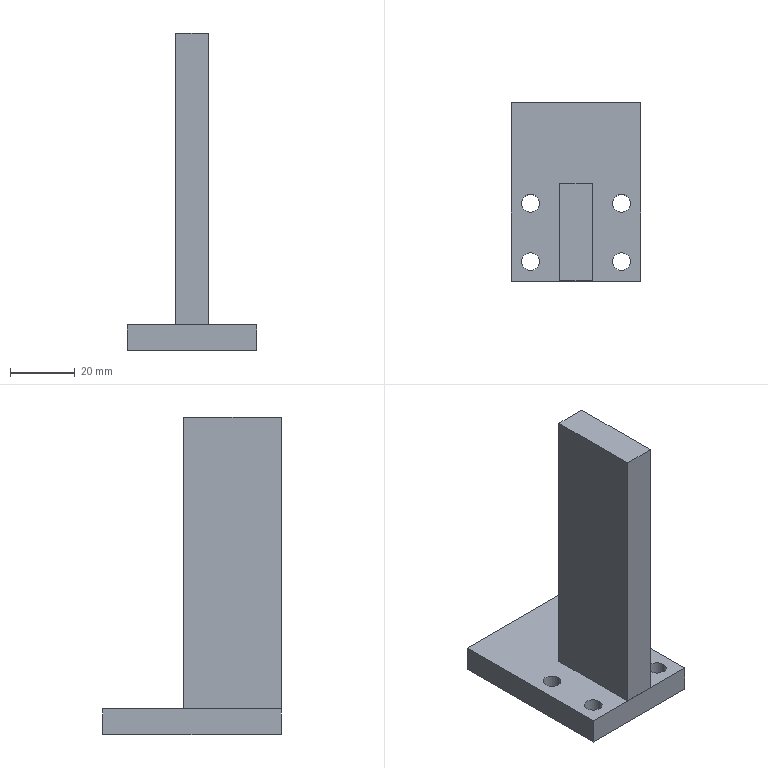Part | STEP file | X77-04020 | 2 solids | 20 faces | box 40 x 55 x 98 mm | volume 43840 mm3 | plane 12 | cylinder 8 | commonest cylinder face diameters 5.5 x8
STEP:
#1=CARTESIAN_POINT('',(338.059,99.5,0.));
#2=VERTEX_POINT('',#1);
#3=CARTESIAN_POINT('',(338.059,129.5,0.));
#4=VERTEX_POINT('',#3);
#5=CARTESIAN_POINT('',(338.059,99.5,0.));
#6=DIRECTION('',(0.,1.,0.));
#7=VECTOR('',#6,1000.);
#8=LINE('',#5,#7);
#9=EDGE_CURVE('',#2,#4,#8,.T.);
#10=ORIENTED_EDGE('',*,*,#9,.T.);
#11=CARTESIAN_POINT('',(338.059,129.5,90.));
#12=VERTEX_POINT('',#11);
#13=CARTESIAN_POINT('',(338.059,129.5,90.));
#14=DIRECTION('',(0.,0.,-1.));
#15=VECTOR('',#14,1000.);
#16=LINE('',#13,#15);
#17=EDGE_CURVE('',#12,#4,#16,.T.);
#18=ORIENTED_EDGE('',*,*,#17,.F.);
#19=CARTESIAN_POINT('',(338.059,99.5,90.));
#20=VERTEX_POINT('',#19);
#21=CARTESIAN_POINT('',(338.059,99.5,90.));
#22=DIRECTION('',(0.,1.,0.));
#23=VECTOR('',#22,1000.);
#24=LINE('',#21,#23);
#25=EDGE_CURVE('',#20,#12,#24,.T.);
#26=ORIENTED_EDGE('',*,*,#25,.F.);
#27=CARTESIAN_POINT('',(338.059,99.5,90.));
#28=DIRECTION('',(0.,0.,-1.));
#29=VECTOR('',#28,1000.);
#30=LINE('',#27,#29);
#31=EDGE_CURVE('',#20,#2,#30,.T.);
#32=ORIENTED_EDGE('',*,*,#31,.T.);
#33=EDGE_LOOP('',(#10,#18,#26,#32));
#34=FACE_OUTER_BOUND('',#33,.T.);
#35=CARTESIAN_POINT('',(338.059,99.5,90.));
#36=DIRECTION('',(-1.,0.,0.));
#37=DIRECTION('',(0.,0.,1.));
#38=AXIS2_PLACEMENT_3D('',#35,#36,#37);
#39=PLANE('',#38);
#40=ADVANCED_FACE('',(#34),#39,.F.);
#41=CARTESIAN_POINT('',(328.059,129.5,0.));
#42=VERTEX_POINT('',#41);
#43=CARTESIAN_POINT('',(328.059,129.5,0.));
#44=DIRECTION('',(-1.,0.,0.));
#45=VECTOR('',#44,1000.);
#46=LINE('',#43,#45);
#47=EDGE_CURVE('',#4,#42,#46,.T.);
#48=ORIENTED_EDGE('',*,*,#47,.T.);
#49=CARTESIAN_POINT('',(328.059,129.5,90.));
#50=VERTEX_POINT('',#49);
#51=CARTESIAN_POINT('',(328.059,129.5,90.));
#52=DIRECTION('',(0.,0.,-1.));
#53=VECTOR('',#52,1000.);
#54=LINE('',#51,#53);
#55=EDGE_CURVE('',#50,#42,#54,.T.);
#56=ORIENTED_EDGE('',*,*,#55,.F.);
#57=CARTESIAN_POINT('',(328.059,129.5,90.));
#58=DIRECTION('',(-1.,0.,0.));
#59=VECTOR('',#58,1000.);
#60=LINE('',#57,#59);
#61=EDGE_CURVE('',#12,#50,#60,.T.);
#62=ORIENTED_EDGE('',*,*,#61,.F.);
#63=ORIENTED_EDGE('',*,*,#17,.T.);
#64=EDGE_LOOP('',(#48,#56,#62,#63));
#65=FACE_OUTER_BOUND('',#64,.T.);
#66=CARTESIAN_POINT('',(328.059,129.5,90.));
#67=DIRECTION('',(0.,-1.,0.));
#68=DIRECTION('',(0.,0.,-1.));
#69=AXIS2_PLACEMENT_3D('',#66,#67,#68);
#70=PLANE('',#69);
#71=ADVANCED_FACE('',(#65),#70,.F.);
#72=CARTESIAN_POINT('',(328.059,99.5,0.));
#73=VERTEX_POINT('',#72);
#74=CARTESIAN_POINT('',(328.059,99.5,0.));
#75=DIRECTION('',(0.,-1.,0.));
#76=VECTOR('',#75,1000.);
#77=LINE('',#74,#76);
#78=EDGE_CURVE('',#42,#73,#77,.T.);
#79=ORIENTED_EDGE('',*,*,#78,.T.);
#80=CARTESIAN_POINT('',(328.059,99.5,90.));
#81=VERTEX_POINT('',#80);
#82=CARTESIAN_POINT('',(328.059,99.5,90.));
#83=DIRECTION('',(0.,0.,-1.));
#84=VECTOR('',#83,1000.);
#85=LINE('',#82,#84);
#86=EDGE_CURVE('',#81,#73,#85,.T.);
#87=ORIENTED_EDGE('',*,*,#86,.F.);
#88=CARTESIAN_POINT('',(328.059,99.5,90.));
#89=DIRECTION('',(0.,-1.,0.));
#90=VECTOR('',#89,1000.);
#91=LINE('',#88,#90);
#92=EDGE_CURVE('',#50,#81,#91,.T.);
#93=ORIENTED_EDGE('',*,*,#92,.F.);
#94=ORIENTED_EDGE('',*,*,#55,.T.);
#95=EDGE_LOOP('',(#79,#87,#93,#94));
#96=FACE_OUTER_BOUND('',#95,.T.);
#97=CARTESIAN_POINT('',(328.059,99.5,90.));
#98=DIRECTION('',(1.,0.,0.));
#99=DIRECTION('',(0.,0.,-1.));
#100=AXIS2_PLACEMENT_3D('',#97,#98,#99);
#101=PLANE('',#100);
#102=ADVANCED_FACE('',(#96),#101,.F.);
#103=CARTESIAN_POINT('',(328.059,99.5,0.));
#104=DIRECTION('',(1.,0.,0.));
#105=VECTOR('',#104,1000.);
#106=LINE('',#103,#105);
#107=EDGE_CURVE('',#73,#2,#106,.T.);
#108=ORIENTED_EDGE('',*,*,#107,.T.);
#109=ORIENTED_EDGE('',*,*,#31,.F.);
#110=CARTESIAN_POINT('',(328.059,99.5,90.));
#111=DIRECTION('',(1.,0.,0.));
#112=VECTOR('',#111,1000.);
#113=LINE('',#110,#112);
#114=EDGE_CURVE('',#81,#20,#113,.T.);
#115=ORIENTED_EDGE('',*,*,#114,.F.);
#116=ORIENTED_EDGE('',*,*,#86,.T.);
#117=EDGE_LOOP('',(#108,#109,#115,#116));
#118=FACE_OUTER_BOUND('',#117,.T.);
#119=CARTESIAN_POINT('',(328.059,99.5,90.));
#120=DIRECTION('',(0.,1.,0.));
#121=DIRECTION('',(0.,0.,1.));
#122=AXIS2_PLACEMENT_3D('',#119,#120,#121);
#123=PLANE('',#122);
#124=ADVANCED_FACE('',(#118),#123,.F.);
#125=ORIENTED_EDGE('',*,*,#25,.T.);
#126=ORIENTED_EDGE('',*,*,#61,.T.);
#127=ORIENTED_EDGE('',*,*,#92,.T.);
#128=ORIENTED_EDGE('',*,*,#114,.T.);
#129=EDGE_LOOP('',(#125,#126,#127,#128));
#130=FACE_OUTER_BOUND('',#129,.T.);
#131=CARTESIAN_POINT('',(338.059,129.5,90.));
#132=DIRECTION('',(0.,0.,-1.));
#133=DIRECTION('',(-1.,0.,0.));
#134=AXIS2_PLACEMENT_3D('',#131,#132,#133);
#135=PLANE('',#134);
#136=ADVANCED_FACE('',(#130),#135,.F.);
#137=ORIENTED_EDGE('',*,*,#9,.F.);
#138=ORIENTED_EDGE('',*,*,#107,.F.);
#139=ORIENTED_EDGE('',*,*,#78,.F.);
#140=ORIENTED_EDGE('',*,*,#47,.F.);
#141=EDGE_LOOP('',(#137,#138,#139,#140));
#142=FACE_OUTER_BOUND('',#141,.T.);
#143=CARTESIAN_POINT('',(338.059,129.5,0.));
#144=DIRECTION('',(0.,0.,-1.));
#145=DIRECTION('',(-1.,0.,0.));
#146=AXIS2_PLACEMENT_3D('',#143,#144,#145);
#147=PLANE('',#146);
#148=ADVANCED_FACE('',(#142),#147,.T.);
#149=CLOSED_SHELL('',(#40,#71,#102,#124,#136,#148));
#150=MANIFOLD_SOLID_BREP('',#149);
#151=CARTESIAN_POINT('',(316.309,123.5,-8.));
#152=VERTEX_POINT('',#151);
#153=CARTESIAN_POINT('',(321.809,123.5,-8.));
#154=VERTEX_POINT('',#153);
#155=CARTESIAN_POINT('',(319.059,123.5,-8.));
#156=DIRECTION('',(0.,0.,1.));
#157=DIRECTION('',(1.,0.,0.));
#158=AXIS2_PLACEMENT_3D('',#155,#156,#157);
#159=CIRCLE('',#158,2.75);
#160=EDGE_CURVE('',#152,#154,#159,.T.);
#161=ORIENTED_EDGE('',*,*,#160,.F.);
#162=CARTESIAN_POINT('',(316.309,123.5,0.));
#163=VERTEX_POINT('',#162);
#164=CARTESIAN_POINT('',(316.309,123.5,0.));
#165=DIRECTION('',(0.,0.,1.));
#166=VECTOR('',#165,1000.);
#167=LINE('',#164,#166);
#168=EDGE_CURVE('',#152,#163,#167,.T.);
#169=ORIENTED_EDGE('',*,*,#168,.T.);
#170=CARTESIAN_POINT('',(321.809,123.5,0.));
#171=VERTEX_POINT('',#170);
#172=CARTESIAN_POINT('',(319.059,123.5,0.));
#173=DIRECTION('',(0.,0.,1.));
#174=DIRECTION('',(1.,0.,0.));
#175=AXIS2_PLACEMENT_3D('',#172,#173,#174);
#176=CIRCLE('',#175,2.75);
#177=EDGE_CURVE('',#163,#171,#176,.T.);
#178=ORIENTED_EDGE('',*,*,#177,.T.);
#179=CARTESIAN_POINT('',(321.809,123.5,0.));
#180=DIRECTION('',(0.,0.,1.));
#181=VECTOR('',#180,1000.);
#182=LINE('',#179,#181);
#183=EDGE_CURVE('',#154,#171,#182,.T.);
#184=ORIENTED_EDGE('',*,*,#183,.F.);
#185=EDGE_LOOP('',(#161,#169,#178,#184));
#186=FACE_OUTER_BOUND('',#185,.T.);
#187=CARTESIAN_POINT('',(319.059,123.5,0.));
#188=DIRECTION('',(0.,0.,1.));
#189=DIRECTION('',(1.,0.,0.));
#190=AXIS2_PLACEMENT_3D('',#187,#188,#189);
#191=CYLINDRICAL_SURFACE('',#190,2.75);
#192=ADVANCED_FACE('',(#186),#191,.F.);
#193=CARTESIAN_POINT('',(344.309,123.5,-8.));
#194=VERTEX_POINT('',#193);
#195=CARTESIAN_POINT('',(349.809,123.5,-8.));
#196=VERTEX_POINT('',#195);
#197=CARTESIAN_POINT('',(347.059,123.5,-8.));
#198=DIRECTION('',(0.,0.,1.));
#199=DIRECTION('',(1.,0.,0.));
#200=AXIS2_PLACEMENT_3D('',#197,#198,#199);
#201=CIRCLE('',#200,2.75);
#202=EDGE_CURVE('',#194,#196,#201,.T.);
#203=ORIENTED_EDGE('',*,*,#202,.F.);
#204=CARTESIAN_POINT('',(344.309,123.5,0.));
#205=VERTEX_POINT('',#204);
#206=CARTESIAN_POINT('',(344.309,123.5,0.));
#207=DIRECTION('',(0.,0.,1.));
#208=VECTOR('',#207,1000.);
#209=LINE('',#206,#208);
#210=EDGE_CURVE('',#194,#205,#209,.T.);
#211=ORIENTED_EDGE('',*,*,#210,.T.);
#212=CARTESIAN_POINT('',(349.809,123.5,0.));
#213=VERTEX_POINT('',#212);
#214=CARTESIAN_POINT('',(347.059,123.5,0.));
#215=DIRECTION('',(0.,0.,1.));
#216=DIRECTION('',(1.,0.,0.));
#217=AXIS2_PLACEMENT_3D('',#214,#215,#216);
#218=CIRCLE('',#217,2.75);
#219=EDGE_CURVE('',#205,#213,#218,.T.);
#220=ORIENTED_EDGE('',*,*,#219,.T.);
#221=CARTESIAN_POINT('',(349.809,123.5,0.));
#222=DIRECTION('',(0.,0.,1.));
#223=VECTOR('',#222,1000.);
#224=LINE('',#221,#223);
#225=EDGE_CURVE('',#196,#213,#224,.T.);
#226=ORIENTED_EDGE('',*,*,#225,.F.);
#227=EDGE_LOOP('',(#203,#211,#220,#226));
#228=FACE_OUTER_BOUND('',#227,.T.);
#229=CARTESIAN_POINT('',(347.059,123.5,0.));
#230=DIRECTION('',(0.,0.,1.));
#231=DIRECTION('',(1.,0.,0.));
#232=AXIS2_PLACEMENT_3D('',#229,#230,#231);
#233=CYLINDRICAL_SURFACE('',#232,2.75);
#234=ADVANCED_FACE('',(#228),#233,.F.);
#235=CARTESIAN_POINT('',(316.309,105.5,-8.));
#236=VERTEX_POINT('',#235);
#237=CARTESIAN_POINT('',(321.809,105.5,-8.));
#238=VERTEX_POINT('',#237);
#239=CARTESIAN_POINT('',(319.059,105.5,-8.));
#240=DIRECTION('',(0.,0.,1.));
#241=DIRECTION('',(1.,0.,0.));
#242=AXIS2_PLACEMENT_3D('',#239,#240,#241);
#243=CIRCLE('',#242,2.75);
#244=EDGE_CURVE('',#236,#238,#243,.T.);
#245=ORIENTED_EDGE('',*,*,#244,.F.);
#246=CARTESIAN_POINT('',(316.309,105.5,0.));
#247=VERTEX_POINT('',#246);
#248=CARTESIAN_POINT('',(316.309,105.5,0.));
#249=DIRECTION('',(0.,0.,1.));
#250=VECTOR('',#249,1000.);
#251=LINE('',#248,#250);
#252=EDGE_CURVE('',#236,#247,#251,.T.);
#253=ORIENTED_EDGE('',*,*,#252,.T.);
#254=CARTESIAN_POINT('',(321.809,105.5,0.));
#255=VERTEX_POINT('',#254);
#256=CARTESIAN_POINT('',(319.059,105.5,0.));
#257=DIRECTION('',(0.,0.,1.));
#258=DIRECTION('',(1.,0.,0.));
#259=AXIS2_PLACEMENT_3D('',#256,#257,#258);
#260=CIRCLE('',#259,2.75);
#261=EDGE_CURVE('',#247,#255,#260,.T.);
#262=ORIENTED_EDGE('',*,*,#261,.T.);
#263=CARTESIAN_POINT('',(321.809,105.5,0.));
#264=DIRECTION('',(0.,0.,1.));
#265=VECTOR('',#264,1000.);
#266=LINE('',#263,#265);
#267=EDGE_CURVE('',#238,#255,#266,.T.);
#268=ORIENTED_EDGE('',*,*,#267,.F.);
#269=EDGE_LOOP('',(#245,#253,#262,#268));
#270=FACE_OUTER_BOUND('',#269,.T.);
#271=CARTESIAN_POINT('',(319.059,105.5,0.));
#272=DIRECTION('',(0.,0.,1.));
#273=DIRECTION('',(1.,0.,0.));
#274=AXIS2_PLACEMENT_3D('',#271,#272,#273);
#275=CYLINDRICAL_SURFACE('',#274,2.75);
#276=ADVANCED_FACE('',(#270),#275,.F.);
#277=CARTESIAN_POINT('',(344.309,105.5,-8.));
#278=VERTEX_POINT('',#277);
#279=CARTESIAN_POINT('',(349.809,105.5,-8.));
#280=VERTEX_POINT('',#279);
#281=CARTESIAN_POINT('',(347.059,105.5,-8.));
#282=DIRECTION('',(0.,0.,1.));
#283=DIRECTION('',(1.,0.,0.));
#284=AXIS2_PLACEMENT_3D('',#281,#282,#283);
#285=CIRCLE('',#284,2.75);
#286=EDGE_CURVE('',#278,#280,#285,.T.);
#287=ORIENTED_EDGE('',*,*,#286,.F.);
#288=CARTESIAN_POINT('',(344.309,105.5,0.));
#289=VERTEX_POINT('',#288);
#290=CARTESIAN_POINT('',(344.309,105.5,0.));
#291=DIRECTION('',(0.,0.,1.));
#292=VECTOR('',#291,1000.);
#293=LINE('',#290,#292);
#294=EDGE_CURVE('',#278,#289,#293,.T.);
#295=ORIENTED_EDGE('',*,*,#294,.T.);
#296=CARTESIAN_POINT('',(349.809,105.5,0.));
#297=VERTEX_POINT('',#296);
#298=CARTESIAN_POINT('',(347.059,105.5,0.));
#299=DIRECTION('',(0.,0.,1.));
#300=DIRECTION('',(1.,0.,0.));
#301=AXIS2_PLACEMENT_3D('',#298,#299,#300);
#302=CIRCLE('',#301,2.75);
#303=EDGE_CURVE('',#289,#297,#302,.T.);
#304=ORIENTED_EDGE('',*,*,#303,.T.);
#305=CARTESIAN_POINT('',(349.809,105.5,0.));
#306=DIRECTION('',(0.,0.,1.));
#307=VECTOR('',#306,1000.);
#308=LINE('',#305,#307);
#309=EDGE_CURVE('',#280,#297,#308,.T.);
#310=ORIENTED_EDGE('',*,*,#309,.F.);
#311=EDGE_LOOP('',(#287,#295,#304,#310));
#312=FACE_OUTER_BOUND('',#311,.T.);
#313=CARTESIAN_POINT('',(347.059,105.5,0.));
#314=DIRECTION('',(0.,0.,1.));
#315=DIRECTION('',(1.,0.,0.));
#316=AXIS2_PLACEMENT_3D('',#313,#314,#315);
#317=CYLINDRICAL_SURFACE('',#316,2.75);
#318=ADVANCED_FACE('',(#312),#317,.F.);
#319=CARTESIAN_POINT('',(313.059,99.5,0.));
#320=VERTEX_POINT('',#319);
#321=CARTESIAN_POINT('',(313.059,154.5,0.));
#322=VERTEX_POINT('',#321);
#323=CARTESIAN_POINT('',(313.059,99.5,0.));
#324=DIRECTION('',(0.,1.,0.));
#325=VECTOR('',#324,1000.);
#326=LINE('',#323,#325);
#327=EDGE_CURVE('',#320,#322,#326,.T.);
#328=ORIENTED_EDGE('',*,*,#327,.T.);
#329=CARTESIAN_POINT('',(313.059,154.5,-8.));
#330=VERTEX_POINT('',#329);
#331=CARTESIAN_POINT('',(313.059,154.5,0.));
#332=DIRECTION('',(0.,0.,1.));
#333=VECTOR('',#332,1000.);
#334=LINE('',#331,#333);
#335=EDGE_CURVE('',#330,#322,#334,.T.);
#336=ORIENTED_EDGE('',*,*,#335,.F.);
#337=CARTESIAN_POINT('',(313.059,99.5,-8.));
#338=VERTEX_POINT('',#337);
#339=CARTESIAN_POINT('',(313.059,99.5,-8.));
#340=DIRECTION('',(0.,1.,0.));
#341=VECTOR('',#340,1000.);
#342=LINE('',#339,#341);
#343=EDGE_CURVE('',#338,#330,#342,.T.);
#344=ORIENTED_EDGE('',*,*,#343,.F.);
#345=CARTESIAN_POINT('',(313.059,99.5,-8.));
#346=DIRECTION('',(0.,0.,1.));
#347=VECTOR('',#346,1000.);
#348=LINE('',#345,#347);
#349=EDGE_CURVE('',#338,#320,#348,.T.);
#350=ORIENTED_EDGE('',*,*,#349,.T.);
#351=EDGE_LOOP('',(#328,#336,#344,#350));
#352=FACE_OUTER_BOUND('',#351,.T.);
#353=CARTESIAN_POINT('',(313.059,99.5,-8.));
#354=DIRECTION('',(1.,0.,0.));
#355=DIRECTION('',(0.,0.,-1.));
#356=AXIS2_PLACEMENT_3D('',#353,#354,#355);
#357=PLANE('',#356);
#358=ADVANCED_FACE('',(#352),#357,.F.);
#359=CARTESIAN_POINT('',(353.059,154.5,0.));
#360=VERTEX_POINT('',#359);
#361=CARTESIAN_POINT('',(353.059,99.5,0.));
#362=VERTEX_POINT('',#361);
#363=CARTESIAN_POINT('',(353.059,99.5,0.));
#364=DIRECTION('',(0.,-1.,0.));
#365=VECTOR('',#364,1000.);
#366=LINE('',#363,#365);
#367=EDGE_CURVE('',#360,#362,#366,.T.);
#368=ORIENTED_EDGE('',*,*,#367,.T.);
#369=CARTESIAN_POINT('',(353.059,99.5,-8.));
#370=VERTEX_POINT('',#369);
#371=CARTESIAN_POINT('',(353.059,99.5,-8.));
#372=DIRECTION('',(0.,0.,1.));
#373=VECTOR('',#372,1000.);
#374=LINE('',#371,#373);
#375=EDGE_CURVE('',#370,#362,#374,.T.);
#376=ORIENTED_EDGE('',*,*,#375,.F.);
#377=CARTESIAN_POINT('',(353.059,154.5,-8.));
#378=VERTEX_POINT('',#377);
#379=CARTESIAN_POINT('',(353.059,99.5,-8.));
#380=DIRECTION('',(0.,-1.,0.));
#381=VECTOR('',#380,1000.);
#382=LINE('',#379,#381);
#383=EDGE_CURVE('',#378,#370,#382,.T.);
#384=ORIENTED_EDGE('',*,*,#383,.F.);
#385=CARTESIAN_POINT('',(353.059,154.5,0.));
#386=DIRECTION('',(0.,0.,-1.));
#387=VECTOR('',#386,1000.);
#388=LINE('',#385,#387);
#389=EDGE_CURVE('',#360,#378,#388,.T.);
#390=ORIENTED_EDGE('',*,*,#389,.F.);
#391=EDGE_LOOP('',(#368,#376,#384,#390));
#392=FACE_OUTER_BOUND('',#391,.T.);
#393=CARTESIAN_POINT('',(353.059,99.5,-8.));
#394=DIRECTION('',(-1.,0.,0.));
#395=DIRECTION('',(0.,0.,1.));
#396=AXIS2_PLACEMENT_3D('',#393,#394,#395);
#397=PLANE('',#396);
#398=ADVANCED_FACE('',(#392),#397,.F.);
#399=CARTESIAN_POINT('',(353.059,99.5,0.));
#400=DIRECTION('',(-1.,0.,0.));
#401=VECTOR('',#400,1000.);
#402=LINE('',#399,#401);
#403=EDGE_CURVE('',#362,#320,#402,.T.);
#404=ORIENTED_EDGE('',*,*,#403,.T.);
#405=ORIENTED_EDGE('',*,*,#349,.F.);
#406=CARTESIAN_POINT('',(353.059,99.5,-8.));
#407=DIRECTION('',(-1.,0.,0.));
#408=VECTOR('',#407,1000.);
#409=LINE('',#406,#408);
#410=EDGE_CURVE('',#370,#338,#409,.T.);
#411=ORIENTED_EDGE('',*,*,#410,.F.);
#412=ORIENTED_EDGE('',*,*,#375,.T.);
#413=EDGE_LOOP('',(#404,#405,#411,#412));
#414=FACE_OUTER_BOUND('',#413,.T.);
#415=CARTESIAN_POINT('',(353.059,99.5,-8.));
#416=DIRECTION('',(0.,1.,0.));
#417=DIRECTION('',(0.,0.,1.));
#418=AXIS2_PLACEMENT_3D('',#415,#416,#417);
#419=PLANE('',#418);
#420=ADVANCED_FACE('',(#414),#419,.F.);
#421=CARTESIAN_POINT('',(319.059,123.5,-8.));
#422=DIRECTION('',(0.,0.,1.));
#423=DIRECTION('',(1.,0.,0.));
#424=AXIS2_PLACEMENT_3D('',#421,#422,#423);
#425=CIRCLE('',#424,2.75);
#426=EDGE_CURVE('',#154,#152,#425,.T.);
#427=ORIENTED_EDGE('',*,*,#426,.T.);
#428=ORIENTED_EDGE('',*,*,#160,.T.);
#429=EDGE_LOOP('',(#427,#428));
#430=FACE_BOUND('',#429,.T.);
#431=CARTESIAN_POINT('',(347.059,123.5,-8.));
#432=DIRECTION('',(0.,0.,1.));
#433=DIRECTION('',(1.,0.,0.));
#434=AXIS2_PLACEMENT_3D('',#431,#432,#433);
#435=CIRCLE('',#434,2.75);
#436=EDGE_CURVE('',#196,#194,#435,.T.);
#437=ORIENTED_EDGE('',*,*,#436,.T.);
#438=ORIENTED_EDGE('',*,*,#202,.T.);
#439=EDGE_LOOP('',(#437,#438));
#440=FACE_BOUND('',#439,.T.);
#441=CARTESIAN_POINT('',(319.059,105.5,-8.));
#442=DIRECTION('',(0.,0.,1.));
#443=DIRECTION('',(1.,0.,0.));
#444=AXIS2_PLACEMENT_3D('',#441,#442,#443);
#445=CIRCLE('',#444,2.75);
#446=EDGE_CURVE('',#238,#236,#445,.T.);
#447=ORIENTED_EDGE('',*,*,#446,.T.);
#448=ORIENTED_EDGE('',*,*,#244,.T.);
#449=EDGE_LOOP('',(#447,#448));
#450=FACE_BOUND('',#449,.T.);
#451=CARTESIAN_POINT('',(347.059,105.5,-8.));
#452=DIRECTION('',(0.,0.,1.));
#453=DIRECTION('',(1.,0.,0.));
#454=AXIS2_PLACEMENT_3D('',#451,#452,#453);
#455=CIRCLE('',#454,2.75);
#456=EDGE_CURVE('',#280,#278,#455,.T.);
#457=ORIENTED_EDGE('',*,*,#456,.T.);
#458=ORIENTED_EDGE('',*,*,#286,.T.);
#459=EDGE_LOOP('',(#457,#458));
#460=FACE_BOUND('',#459,.T.);
#461=ORIENTED_EDGE('',*,*,#343,.T.);
#462=CARTESIAN_POINT('',(313.059,154.5,-8.));
#463=DIRECTION('',(-1.,0.,0.));
#464=VECTOR('',#463,1000.);
#465=LINE('',#462,#464);
#466=EDGE_CURVE('',#378,#330,#465,.T.);
#467=ORIENTED_EDGE('',*,*,#466,.F.);
#468=ORIENTED_EDGE('',*,*,#383,.T.);
#469=ORIENTED_EDGE('',*,*,#410,.T.);
#470=EDGE_LOOP('',(#461,#467,#468,#469));
#471=FACE_OUTER_BOUND('',#470,.T.);
#472=CARTESIAN_POINT('',(313.059,129.5,-8.));
#473=DIRECTION('',(0.,0.,1.));
#474=DIRECTION('',(1.,0.,0.));
#475=AXIS2_PLACEMENT_3D('',#472,#473,#474);
#476=PLANE('',#475);
#477=ADVANCED_FACE('',(#430,#440,#450,#460,#471),#476,.F.);
#478=CARTESIAN_POINT('',(319.059,123.5,0.));
#479=DIRECTION('',(0.,0.,1.));
#480=DIRECTION('',(1.,0.,0.));
#481=AXIS2_PLACEMENT_3D('',#478,#479,#480);
#482=CIRCLE('',#481,2.75);
#483=EDGE_CURVE('',#171,#163,#482,.T.);
#484=ORIENTED_EDGE('',*,*,#483,.F.);
#485=ORIENTED_EDGE('',*,*,#177,.F.);
#486=EDGE_LOOP('',(#484,#485));
#487=FACE_BOUND('',#486,.T.);
#488=CARTESIAN_POINT('',(347.059,123.5,0.));
#489=DIRECTION('',(0.,0.,1.));
#490=DIRECTION('',(1.,0.,0.));
#491=AXIS2_PLACEMENT_3D('',#488,#489,#490);
#492=CIRCLE('',#491,2.75);
#493=EDGE_CURVE('',#213,#205,#492,.T.);
#494=ORIENTED_EDGE('',*,*,#493,.F.);
#495=ORIENTED_EDGE('',*,*,#219,.F.);
#496=EDGE_LOOP('',(#494,#495));
#497=FACE_BOUND('',#496,.T.);
#498=CARTESIAN_POINT('',(319.059,105.5,0.));
#499=DIRECTION('',(0.,0.,1.));
#500=DIRECTION('',(1.,0.,0.));
#501=AXIS2_PLACEMENT_3D('',#498,#499,#500);
#502=CIRCLE('',#501,2.75);
#503=EDGE_CURVE('',#255,#247,#502,.T.);
#504=ORIENTED_EDGE('',*,*,#503,.F.);
#505=ORIENTED_EDGE('',*,*,#261,.F.);
#506=EDGE_LOOP('',(#504,#505));
#507=FACE_BOUND('',#506,.T.);
#508=CARTESIAN_POINT('',(347.059,105.5,0.));
#509=DIRECTION('',(0.,0.,1.));
#510=DIRECTION('',(1.,0.,0.));
#511=AXIS2_PLACEMENT_3D('',#508,#509,#510);
#512=CIRCLE('',#511,2.75);
#513=EDGE_CURVE('',#297,#289,#512,.T.);
#514=ORIENTED_EDGE('',*,*,#513,.F.);
#515=ORIENTED_EDGE('',*,*,#303,.F.);
#516=EDGE_LOOP('',(#514,#515));
#517=FACE_BOUND('',#516,.T.);
#518=ORIENTED_EDGE('',*,*,#327,.F.);
#519=ORIENTED_EDGE('',*,*,#403,.F.);
#520=ORIENTED_EDGE('',*,*,#367,.F.);
#521=CARTESIAN_POINT('',(313.059,154.5,0.));
#522=DIRECTION('',(1.,0.,0.));
#523=VECTOR('',#522,1000.);
#524=LINE('',#521,#523);
#525=EDGE_CURVE('',#322,#360,#524,.T.);
#526=ORIENTED_EDGE('',*,*,#525,.F.);
#527=EDGE_LOOP('',(#518,#519,#520,#526));
#528=FACE_OUTER_BOUND('',#527,.T.);
#529=CARTESIAN_POINT('',(313.059,129.5,0.));
#530=DIRECTION('',(0.,0.,1.));
#531=DIRECTION('',(1.,0.,0.));
#532=AXIS2_PLACEMENT_3D('',#529,#530,#531);
#533=PLANE('',#532);
#534=ADVANCED_FACE('',(#487,#497,#507,#517,#528),#533,.T.);
#535=ORIENTED_EDGE('',*,*,#294,.F.);
#536=ORIENTED_EDGE('',*,*,#456,.F.);
#537=ORIENTED_EDGE('',*,*,#309,.T.);
#538=ORIENTED_EDGE('',*,*,#513,.T.);
#539=EDGE_LOOP('',(#535,#536,#537,#538));
#540=FACE_OUTER_BOUND('',#539,.T.);
#541=CARTESIAN_POINT('',(347.059,105.5,0.));
#542=DIRECTION('',(0.,0.,1.));
#543=DIRECTION('',(1.,0.,0.));
#544=AXIS2_PLACEMENT_3D('',#541,#542,#543);
#545=CYLINDRICAL_SURFACE('',#544,2.75);
#546=ADVANCED_FACE('',(#540),#545,.F.);
#547=ORIENTED_EDGE('',*,*,#252,.F.);
#548=ORIENTED_EDGE('',*,*,#446,.F.);
#549=ORIENTED_EDGE('',*,*,#267,.T.);
#550=ORIENTED_EDGE('',*,*,#503,.T.);
#551=EDGE_LOOP('',(#547,#548,#549,#550));
#552=FACE_OUTER_BOUND('',#551,.T.);
#553=CARTESIAN_POINT('',(319.059,105.5,0.));
#554=DIRECTION('',(0.,0.,1.));
#555=DIRECTION('',(1.,0.,0.));
#556=AXIS2_PLACEMENT_3D('',#553,#554,#555);
#557=CYLINDRICAL_SURFACE('',#556,2.75);
#558=ADVANCED_FACE('',(#552),#557,.F.);
#559=ORIENTED_EDGE('',*,*,#210,.F.);
#560=ORIENTED_EDGE('',*,*,#436,.F.);
#561=ORIENTED_EDGE('',*,*,#225,.T.);
#562=ORIENTED_EDGE('',*,*,#493,.T.);
#563=EDGE_LOOP('',(#559,#560,#561,#562));
#564=FACE_OUTER_BOUND('',#563,.T.);
#565=CARTESIAN_POINT('',(347.059,123.5,0.));
#566=DIRECTION('',(0.,0.,1.));
#567=DIRECTION('',(1.,0.,0.));
#568=AXIS2_PLACEMENT_3D('',#565,#566,#567);
#569=CYLINDRICAL_SURFACE('',#568,2.75);
#570=ADVANCED_FACE('',(#564),#569,.F.);
#571=ORIENTED_EDGE('',*,*,#168,.F.);
#572=ORIENTED_EDGE('',*,*,#426,.F.);
#573=ORIENTED_EDGE('',*,*,#183,.T.);
#574=ORIENTED_EDGE('',*,*,#483,.T.);
#575=EDGE_LOOP('',(#571,#572,#573,#574));
#576=FACE_OUTER_BOUND('',#575,.T.);
#577=CARTESIAN_POINT('',(319.059,123.5,0.));
#578=DIRECTION('',(0.,0.,1.));
#579=DIRECTION('',(1.,0.,0.));
#580=AXIS2_PLACEMENT_3D('',#577,#578,#579);
#581=CYLINDRICAL_SURFACE('',#580,2.75);
#582=ADVANCED_FACE('',(#576),#581,.F.);
#583=ORIENTED_EDGE('',*,*,#335,.T.);
#584=ORIENTED_EDGE('',*,*,#525,.T.);
#585=ORIENTED_EDGE('',*,*,#389,.T.);
#586=ORIENTED_EDGE('',*,*,#466,.T.);
#587=EDGE_LOOP('',(#583,#584,#585,#586));
#588=FACE_OUTER_BOUND('',#587,.T.);
#589=CARTESIAN_POINT('',(313.059,154.5,-8.));
#590=DIRECTION('',(0.,-1.,0.));
#591=DIRECTION('',(0.,0.,-1.));
#592=AXIS2_PLACEMENT_3D('',#589,#590,#591);
#593=PLANE('',#592);
#594=ADVANCED_FACE('',(#588),#593,.F.);
#595=CLOSED_SHELL('',(#192,#234,#276,#318,#358,#398,#420,#477,#534,#546,#558,#570,#582,#594));
#596=MANIFOLD_SOLID_BREP('',#595);
#597=CARTESIAN_POINT('',(0.,0.,0.));
#598=DIRECTION('',(0.,0.,1.));
#599=DIRECTION('',(1.,0.,0.));
#600=AXIS2_PLACEMENT_3D('',#597,#598,#599);
#601=(LENGTH_UNIT()NAMED_UNIT(*)SI_UNIT(.MILLI.,.METRE.));
#602=UNCERTAINTY_MEASURE_WITH_UNIT(LENGTH_MEASURE(0.00001),#601,'','');
#603=(NAMED_UNIT(*)PLANE_ANGLE_UNIT()SI_UNIT($,.RADIAN.));
#604=(NAMED_UNIT(*)SI_UNIT($,.STERADIAN.)SOLID_ANGLE_UNIT());
#605=(GEOMETRIC_REPRESENTATION_CONTEXT(3)GLOBAL_UNCERTAINTY_ASSIGNED_CONTEXT((#602))GLOBAL_UNIT_ASSIGNED_CONTEXT((#601,#603,#604))REPRESENTATION_CONTEXT('',''));
#606=ADVANCED_BREP_SHAPE_REPRESENTATION('',(#150,#596,#600),#605);